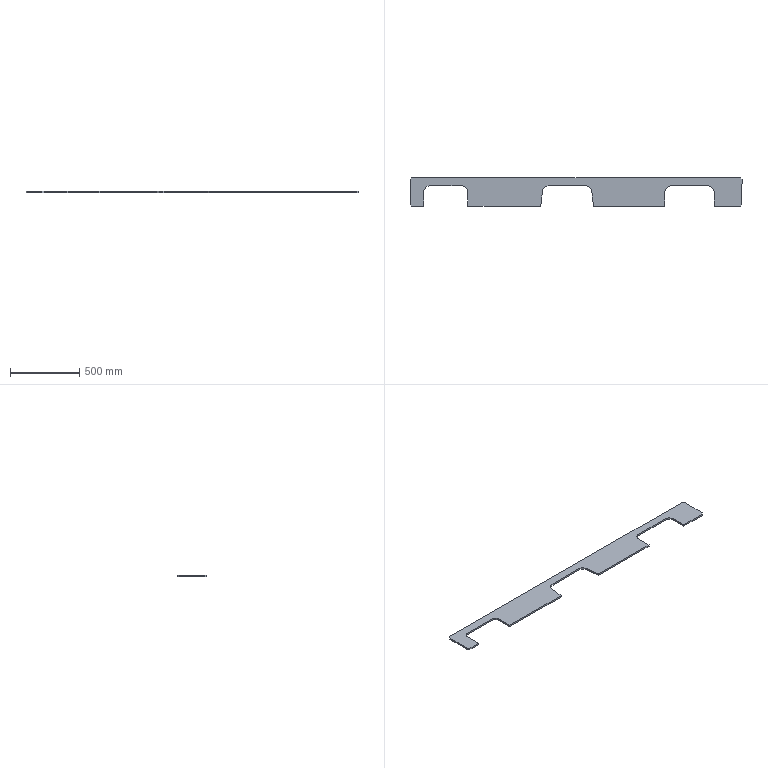Part | SolidWorks | features Extrusion 1 | 1 solid | 28 faces | box 2400 x 207 x 12 mm | volume 4150722 mm3 | plane 22 | cylinder 6 | commonest cylinder face diameters 80 x6
STEP:
#1=CARTESIAN_POINT('',(0.,12.,0.));
#2=VERTEX_POINT('',#1);
#3=CARTESIAN_POINT('',(12.,0.,0.));
#4=VERTEX_POINT('',#3);
#5=CARTESIAN_POINT('',(0.,12.,0.));
#6=DIRECTION('',(0.7071,-0.7071,0.));
#7=VECTOR('',#6,1000.);
#8=LINE('',#5,#7);
#9=EDGE_CURVE('',#2,#4,#8,.T.);
#10=ORIENTED_EDGE('',*,*,#9,.T.);
#11=CARTESIAN_POINT('',(12.,0.,12.));
#12=VERTEX_POINT('',#11);
#13=CARTESIAN_POINT('',(12.,0.,12.));
#14=DIRECTION('',(0.,0.,-1.));
#15=VECTOR('',#14,1000.);
#16=LINE('',#13,#15);
#17=EDGE_CURVE('',#12,#4,#16,.T.);
#18=ORIENTED_EDGE('',*,*,#17,.F.);
#19=CARTESIAN_POINT('',(0.,12.,12.));
#20=VERTEX_POINT('',#19);
#21=CARTESIAN_POINT('',(0.,12.,12.));
#22=DIRECTION('',(0.7071,-0.7071,0.));
#23=VECTOR('',#22,1000.);
#24=LINE('',#21,#23);
#25=EDGE_CURVE('',#20,#12,#24,.T.);
#26=ORIENTED_EDGE('',*,*,#25,.F.);
#27=CARTESIAN_POINT('',(0.,12.,12.));
#28=DIRECTION('',(0.,0.,-1.));
#29=VECTOR('',#28,1000.);
#30=LINE('',#27,#29);
#31=EDGE_CURVE('',#20,#2,#30,.T.);
#32=ORIENTED_EDGE('',*,*,#31,.T.);
#33=EDGE_LOOP('',(#10,#18,#26,#32));
#34=FACE_OUTER_BOUND('',#33,.T.);
#35=CARTESIAN_POINT('',(0.,12.,12.));
#36=DIRECTION('',(0.7071,0.7071,0.));
#37=DIRECTION('',(-0.7071,0.7071,0.));
#38=AXIS2_PLACEMENT_3D('',#35,#36,#37);
#39=PLANE('',#38);
#40=ADVANCED_FACE('',(#34),#39,.F.);
#41=CARTESIAN_POINT('',(100.,0.,0.));
#42=VERTEX_POINT('',#41);
#43=CARTESIAN_POINT('',(12.,0.,0.));
#44=DIRECTION('',(1.,0.,0.));
#45=VECTOR('',#44,1000.);
#46=LINE('',#43,#45);
#47=EDGE_CURVE('',#4,#42,#46,.T.);
#48=ORIENTED_EDGE('',*,*,#47,.T.);
#49=CARTESIAN_POINT('',(100.,0.,12.));
#50=VERTEX_POINT('',#49);
#51=CARTESIAN_POINT('',(100.,0.,12.));
#52=DIRECTION('',(0.,0.,-1.));
#53=VECTOR('',#52,1000.);
#54=LINE('',#51,#53);
#55=EDGE_CURVE('',#50,#42,#54,.T.);
#56=ORIENTED_EDGE('',*,*,#55,.F.);
#57=CARTESIAN_POINT('',(12.,0.,12.));
#58=DIRECTION('',(1.,0.,0.));
#59=VECTOR('',#58,1000.);
#60=LINE('',#57,#59);
#61=EDGE_CURVE('',#12,#50,#60,.T.);
#62=ORIENTED_EDGE('',*,*,#61,.F.);
#63=ORIENTED_EDGE('',*,*,#17,.T.);
#64=EDGE_LOOP('',(#48,#56,#62,#63));
#65=FACE_OUTER_BOUND('',#64,.T.);
#66=CARTESIAN_POINT('',(12.,0.,12.));
#67=DIRECTION('',(0.,1.,0.));
#68=DIRECTION('',(0.,0.,1.));
#69=AXIS2_PLACEMENT_3D('',#66,#67,#68);
#70=PLANE('',#69);
#71=ADVANCED_FACE('',(#65),#70,.F.);
#72=CARTESIAN_POINT('',(100.,107.,0.));
#73=VERTEX_POINT('',#72);
#74=CARTESIAN_POINT('',(100.,107.,0.));
#75=DIRECTION('',(0.,1.,0.));
#76=VECTOR('',#75,1000.);
#77=LINE('',#74,#76);
#78=EDGE_CURVE('',#42,#73,#77,.T.);
#79=ORIENTED_EDGE('',*,*,#78,.T.);
#80=CARTESIAN_POINT('',(100.,107.,12.));
#81=VERTEX_POINT('',#80);
#82=CARTESIAN_POINT('',(100.,107.,12.));
#83=DIRECTION('',(0.,0.,-1.));
#84=VECTOR('',#83,1000.);
#85=LINE('',#82,#84);
#86=EDGE_CURVE('',#81,#73,#85,.T.);
#87=ORIENTED_EDGE('',*,*,#86,.F.);
#88=CARTESIAN_POINT('',(100.,107.,12.));
#89=DIRECTION('',(0.,1.,0.));
#90=VECTOR('',#89,1000.);
#91=LINE('',#88,#90);
#92=EDGE_CURVE('',#50,#81,#91,.T.);
#93=ORIENTED_EDGE('',*,*,#92,.F.);
#94=ORIENTED_EDGE('',*,*,#55,.T.);
#95=EDGE_LOOP('',(#79,#87,#93,#94));
#96=FACE_OUTER_BOUND('',#95,.T.);
#97=CARTESIAN_POINT('',(100.,107.,12.));
#98=DIRECTION('',(-1.,0.,0.));
#99=DIRECTION('',(0.,-1.,0.));
#100=AXIS2_PLACEMENT_3D('',#97,#98,#99);
#101=PLANE('',#100);
#102=ADVANCED_FACE('',(#96),#101,.F.);
#103=CARTESIAN_POINT('',(140.,147.,0.));
#104=VERTEX_POINT('',#103);
#105=CARTESIAN_POINT('',(140.,107.,0.));
#106=DIRECTION('',(0.,0.,-1.));
#107=DIRECTION('',(-1.,0.,0.));
#108=AXIS2_PLACEMENT_3D('',#105,#106,#107);
#109=CIRCLE('',#108,40.);
#110=EDGE_CURVE('',#73,#104,#109,.T.);
#111=ORIENTED_EDGE('',*,*,#110,.T.);
#112=CARTESIAN_POINT('',(140.,147.,12.));
#113=VERTEX_POINT('',#112);
#114=CARTESIAN_POINT('',(140.,147.,12.));
#115=DIRECTION('',(0.,0.,-1.));
#116=VECTOR('',#115,1000.);
#117=LINE('',#114,#116);
#118=EDGE_CURVE('',#113,#104,#117,.T.);
#119=ORIENTED_EDGE('',*,*,#118,.F.);
#120=CARTESIAN_POINT('',(140.,107.,12.));
#121=DIRECTION('',(0.,0.,-1.));
#122=DIRECTION('',(-1.,0.,0.));
#123=AXIS2_PLACEMENT_3D('',#120,#121,#122);
#124=CIRCLE('',#123,40.);
#125=EDGE_CURVE('',#81,#113,#124,.T.);
#126=ORIENTED_EDGE('',*,*,#125,.F.);
#127=ORIENTED_EDGE('',*,*,#86,.T.);
#128=EDGE_LOOP('',(#111,#119,#126,#127));
#129=FACE_OUTER_BOUND('',#128,.T.);
#130=CARTESIAN_POINT('',(140.,107.,12.));
#131=DIRECTION('',(0.,0.,-1.));
#132=DIRECTION('',(-1.,0.,0.));
#133=AXIS2_PLACEMENT_3D('',#130,#131,#132);
#134=CYLINDRICAL_SURFACE('',#133,40.);
#135=ADVANCED_FACE('',(#129),#134,.F.);
#136=CARTESIAN_POINT('',(378.,147.,0.));
#137=VERTEX_POINT('',#136);
#138=CARTESIAN_POINT('',(140.,147.,0.));
#139=DIRECTION('',(1.,0.,0.));
#140=VECTOR('',#139,1000.);
#141=LINE('',#138,#140);
#142=EDGE_CURVE('',#104,#137,#141,.T.);
#143=ORIENTED_EDGE('',*,*,#142,.T.);
#144=CARTESIAN_POINT('',(378.,147.,12.));
#145=VERTEX_POINT('',#144);
#146=CARTESIAN_POINT('',(378.,147.,12.));
#147=DIRECTION('',(0.,0.,-1.));
#148=VECTOR('',#147,1000.);
#149=LINE('',#146,#148);
#150=EDGE_CURVE('',#145,#137,#149,.T.);
#151=ORIENTED_EDGE('',*,*,#150,.F.);
#152=CARTESIAN_POINT('',(140.,147.,12.));
#153=DIRECTION('',(1.,0.,0.));
#154=VECTOR('',#153,1000.);
#155=LINE('',#152,#154);
#156=EDGE_CURVE('',#113,#145,#155,.T.);
#157=ORIENTED_EDGE('',*,*,#156,.F.);
#158=ORIENTED_EDGE('',*,*,#118,.T.);
#159=EDGE_LOOP('',(#143,#151,#157,#158));
#160=FACE_OUTER_BOUND('',#159,.T.);
#161=CARTESIAN_POINT('',(140.,147.,12.));
#162=DIRECTION('',(0.,1.,0.));
#163=DIRECTION('',(-1.,0.,0.));
#164=AXIS2_PLACEMENT_3D('',#161,#162,#163);
#165=PLANE('',#164);
#166=ADVANCED_FACE('',(#160),#165,.F.);
#167=CARTESIAN_POINT('',(418.,107.,0.));
#168=VERTEX_POINT('',#167);
#169=CARTESIAN_POINT('',(378.,107.,0.));
#170=DIRECTION('',(0.,0.,-1.));
#171=DIRECTION('',(1.,0.,0.));
#172=AXIS2_PLACEMENT_3D('',#169,#170,#171);
#173=CIRCLE('',#172,40.);
#174=EDGE_CURVE('',#137,#168,#173,.T.);
#175=ORIENTED_EDGE('',*,*,#174,.T.);
#176=CARTESIAN_POINT('',(418.,107.,12.));
#177=VERTEX_POINT('',#176);
#178=CARTESIAN_POINT('',(418.,107.,12.));
#179=DIRECTION('',(0.,0.,-1.));
#180=VECTOR('',#179,1000.);
#181=LINE('',#178,#180);
#182=EDGE_CURVE('',#177,#168,#181,.T.);
#183=ORIENTED_EDGE('',*,*,#182,.F.);
#184=CARTESIAN_POINT('',(378.,107.,12.));
#185=DIRECTION('',(0.,0.,-1.));
#186=DIRECTION('',(1.,0.,0.));
#187=AXIS2_PLACEMENT_3D('',#184,#185,#186);
#188=CIRCLE('',#187,40.);
#189=EDGE_CURVE('',#145,#177,#188,.T.);
#190=ORIENTED_EDGE('',*,*,#189,.F.);
#191=ORIENTED_EDGE('',*,*,#150,.T.);
#192=EDGE_LOOP('',(#175,#183,#190,#191));
#193=FACE_OUTER_BOUND('',#192,.T.);
#194=CARTESIAN_POINT('',(378.,107.,12.));
#195=DIRECTION('',(0.,0.,-1.));
#196=DIRECTION('',(-1.,0.,0.));
#197=AXIS2_PLACEMENT_3D('',#194,#195,#196);
#198=CYLINDRICAL_SURFACE('',#197,40.);
#199=ADVANCED_FACE('',(#193),#198,.F.);
#200=CARTESIAN_POINT('',(418.,0.,0.));
#201=VERTEX_POINT('',#200);
#202=CARTESIAN_POINT('',(418.,107.,0.));
#203=DIRECTION('',(0.,-1.,0.));
#204=VECTOR('',#203,1000.);
#205=LINE('',#202,#204);
#206=EDGE_CURVE('',#168,#201,#205,.T.);
#207=ORIENTED_EDGE('',*,*,#206,.T.);
#208=CARTESIAN_POINT('',(418.,0.,12.));
#209=VERTEX_POINT('',#208);
#210=CARTESIAN_POINT('',(418.,0.,12.));
#211=DIRECTION('',(0.,0.,-1.));
#212=VECTOR('',#211,1000.);
#213=LINE('',#210,#212);
#214=EDGE_CURVE('',#209,#201,#213,.T.);
#215=ORIENTED_EDGE('',*,*,#214,.F.);
#216=CARTESIAN_POINT('',(418.,107.,12.));
#217=DIRECTION('',(0.,-1.,0.));
#218=VECTOR('',#217,1000.);
#219=LINE('',#216,#218);
#220=EDGE_CURVE('',#177,#209,#219,.T.);
#221=ORIENTED_EDGE('',*,*,#220,.F.);
#222=ORIENTED_EDGE('',*,*,#182,.T.);
#223=EDGE_LOOP('',(#207,#215,#221,#222));
#224=FACE_OUTER_BOUND('',#223,.T.);
#225=CARTESIAN_POINT('',(418.,107.,12.));
#226=DIRECTION('',(1.,0.,0.));
#227=DIRECTION('',(0.,0.,-1.));
#228=AXIS2_PLACEMENT_3D('',#225,#226,#227);
#229=PLANE('',#228);
#230=ADVANCED_FACE('',(#224),#229,.F.);
#231=CARTESIAN_POINT('',(944.5,0.,0.));
#232=VERTEX_POINT('',#231);
#233=CARTESIAN_POINT('',(418.,0.,0.));
#234=DIRECTION('',(1.,0.,0.));
#235=VECTOR('',#234,1000.);
#236=LINE('',#233,#235);
#237=EDGE_CURVE('',#201,#232,#236,.T.);
#238=ORIENTED_EDGE('',*,*,#237,.T.);
#239=CARTESIAN_POINT('',(944.5,0.,12.));
#240=VERTEX_POINT('',#239);
#241=CARTESIAN_POINT('',(944.5,0.,12.));
#242=DIRECTION('',(0.,0.,-1.));
#243=VECTOR('',#242,1000.);
#244=LINE('',#241,#243);
#245=EDGE_CURVE('',#240,#232,#244,.T.);
#246=ORIENTED_EDGE('',*,*,#245,.F.);
#247=CARTESIAN_POINT('',(418.,0.,12.));
#248=DIRECTION('',(1.,0.,0.));
#249=VECTOR('',#248,1000.);
#250=LINE('',#247,#249);
#251=EDGE_CURVE('',#209,#240,#250,.T.);
#252=ORIENTED_EDGE('',*,*,#251,.F.);
#253=ORIENTED_EDGE('',*,*,#214,.T.);
#254=EDGE_LOOP('',(#238,#246,#252,#253));
#255=FACE_OUTER_BOUND('',#254,.T.);
#256=CARTESIAN_POINT('',(418.,0.,12.));
#257=DIRECTION('',(0.,1.,0.));
#258=DIRECTION('',(0.,0.,1.));
#259=AXIS2_PLACEMENT_3D('',#256,#257,#258);
#260=PLANE('',#259);
#261=ADVANCED_FACE('',(#255),#260,.F.);
#262=CARTESIAN_POINT('',(958.236,111.875,0.));
#263=VERTEX_POINT('',#262);
#264=CARTESIAN_POINT('',(944.5,0.,0.));
#265=DIRECTION('',(0.1219,0.9925,0.));
#266=VECTOR('',#265,1000.);
#267=LINE('',#264,#266);
#268=EDGE_CURVE('',#232,#263,#267,.T.);
#269=ORIENTED_EDGE('',*,*,#268,.T.);
#270=CARTESIAN_POINT('',(958.236,111.875,12.));
#271=VERTEX_POINT('',#270);
#272=CARTESIAN_POINT('',(958.236,111.875,12.));
#273=DIRECTION('',(0.,0.,-1.));
#274=VECTOR('',#273,1000.);
#275=LINE('',#272,#274);
#276=EDGE_CURVE('',#271,#263,#275,.T.);
#277=ORIENTED_EDGE('',*,*,#276,.F.);
#278=CARTESIAN_POINT('',(944.5,0.,12.));
#279=DIRECTION('',(0.1219,0.9925,0.));
#280=VECTOR('',#279,1000.);
#281=LINE('',#278,#280);
#282=EDGE_CURVE('',#240,#271,#281,.T.);
#283=ORIENTED_EDGE('',*,*,#282,.F.);
#284=ORIENTED_EDGE('',*,*,#245,.T.);
#285=EDGE_LOOP('',(#269,#277,#283,#284));
#286=FACE_OUTER_BOUND('',#285,.T.);
#287=CARTESIAN_POINT('',(944.5,0.,12.));
#288=DIRECTION('',(-0.9925,0.1219,0.));
#289=DIRECTION('',(-0.1219,-0.9925,0.));
#290=AXIS2_PLACEMENT_3D('',#287,#288,#289);
#291=PLANE('',#290);
#292=ADVANCED_FACE('',(#286),#291,.F.);
#293=CARTESIAN_POINT('',(997.938,147.,0.));
#294=VERTEX_POINT('',#293);
#295=CARTESIAN_POINT('',(997.938,107.,0.));
#296=DIRECTION('',(0.,0.,-1.));
#297=DIRECTION('',(-1.,0.,0.));
#298=AXIS2_PLACEMENT_3D('',#295,#296,#297);
#299=CIRCLE('',#298,40.);
#300=EDGE_CURVE('',#263,#294,#299,.T.);
#301=ORIENTED_EDGE('',*,*,#300,.T.);
#302=CARTESIAN_POINT('',(997.938,147.,12.));
#303=VERTEX_POINT('',#302);
#304=CARTESIAN_POINT('',(997.938,147.,12.));
#305=DIRECTION('',(0.,0.,-1.));
#306=VECTOR('',#305,1000.);
#307=LINE('',#304,#306);
#308=EDGE_CURVE('',#303,#294,#307,.T.);
#309=ORIENTED_EDGE('',*,*,#308,.F.);
#310=CARTESIAN_POINT('',(997.938,107.,12.));
#311=DIRECTION('',(0.,0.,-1.));
#312=DIRECTION('',(-1.,0.,0.));
#313=AXIS2_PLACEMENT_3D('',#310,#311,#312);
#314=CIRCLE('',#313,40.);
#315=EDGE_CURVE('',#271,#303,#314,.T.);
#316=ORIENTED_EDGE('',*,*,#315,.F.);
#317=ORIENTED_EDGE('',*,*,#276,.T.);
#318=EDGE_LOOP('',(#301,#309,#316,#317));
#319=FACE_OUTER_BOUND('',#318,.T.);
#320=CARTESIAN_POINT('',(997.938,107.,12.));
#321=DIRECTION('',(0.,0.,-1.));
#322=DIRECTION('',(-1.,0.,0.));
#323=AXIS2_PLACEMENT_3D('',#320,#321,#322);
#324=CYLINDRICAL_SURFACE('',#323,40.);
#325=ADVANCED_FACE('',(#319),#324,.F.);
#326=CARTESIAN_POINT('',(1273.562,147.,0.));
#327=VERTEX_POINT('',#326);
#328=CARTESIAN_POINT('',(997.938,147.,0.));
#329=DIRECTION('',(1.,0.,0.));
#330=VECTOR('',#329,1000.);
#331=LINE('',#328,#330);
#332=EDGE_CURVE('',#294,#327,#331,.T.);
#333=ORIENTED_EDGE('',*,*,#332,.T.);
#334=CARTESIAN_POINT('',(1273.562,147.,12.));
#335=VERTEX_POINT('',#334);
#336=CARTESIAN_POINT('',(1273.562,147.,12.));
#337=DIRECTION('',(0.,0.,-1.));
#338=VECTOR('',#337,1000.);
#339=LINE('',#336,#338);
#340=EDGE_CURVE('',#335,#327,#339,.T.);
#341=ORIENTED_EDGE('',*,*,#340,.F.);
#342=CARTESIAN_POINT('',(997.938,147.,12.));
#343=DIRECTION('',(1.,0.,0.));
#344=VECTOR('',#343,1000.);
#345=LINE('',#342,#344);
#346=EDGE_CURVE('',#303,#335,#345,.T.);
#347=ORIENTED_EDGE('',*,*,#346,.F.);
#348=ORIENTED_EDGE('',*,*,#308,.T.);
#349=EDGE_LOOP('',(#333,#341,#347,#348));
#350=FACE_OUTER_BOUND('',#349,.T.);
#351=CARTESIAN_POINT('',(997.938,147.,12.));
#352=DIRECTION('',(0.,1.,0.));
#353=DIRECTION('',(-1.,0.,0.));
#354=AXIS2_PLACEMENT_3D('',#351,#352,#353);
#355=PLANE('',#354);
#356=ADVANCED_FACE('',(#350),#355,.F.);
#357=CARTESIAN_POINT('',(1313.264,111.875,0.));
#358=VERTEX_POINT('',#357);
#359=CARTESIAN_POINT('',(1273.562,107.,0.));
#360=DIRECTION('',(0.,0.,-1.));
#361=DIRECTION('',(1.,0.,0.));
#362=AXIS2_PLACEMENT_3D('',#359,#360,#361);
#363=CIRCLE('',#362,40.);
#364=EDGE_CURVE('',#327,#358,#363,.T.);
#365=ORIENTED_EDGE('',*,*,#364,.T.);
#366=CARTESIAN_POINT('',(1313.264,111.875,12.));
#367=VERTEX_POINT('',#366);
#368=CARTESIAN_POINT('',(1313.264,111.875,12.));
#369=DIRECTION('',(0.,0.,-1.));
#370=VECTOR('',#369,1000.);
#371=LINE('',#368,#370);
#372=EDGE_CURVE('',#367,#358,#371,.T.);
#373=ORIENTED_EDGE('',*,*,#372,.F.);
#374=CARTESIAN_POINT('',(1273.562,107.,12.));
#375=DIRECTION('',(0.,0.,-1.));
#376=DIRECTION('',(1.,0.,0.));
#377=AXIS2_PLACEMENT_3D('',#374,#375,#376);
#378=CIRCLE('',#377,40.);
#379=EDGE_CURVE('',#335,#367,#378,.T.);
#380=ORIENTED_EDGE('',*,*,#379,.F.);
#381=ORIENTED_EDGE('',*,*,#340,.T.);
#382=EDGE_LOOP('',(#365,#373,#380,#381));
#383=FACE_OUTER_BOUND('',#382,.T.);
#384=CARTESIAN_POINT('',(1273.562,107.,12.));
#385=DIRECTION('',(0.,0.,-1.));
#386=DIRECTION('',(-1.,0.,0.));
#387=AXIS2_PLACEMENT_3D('',#384,#385,#386);
#388=CYLINDRICAL_SURFACE('',#387,40.);
#389=ADVANCED_FACE('',(#383),#388,.F.);
#390=CARTESIAN_POINT('',(1327.,0.,0.));
#391=VERTEX_POINT('',#390);
#392=CARTESIAN_POINT('',(1327.,0.,0.));
#393=DIRECTION('',(0.1219,-0.9925,0.));
#394=VECTOR('',#393,1000.);
#395=LINE('',#392,#394);
#396=EDGE_CURVE('',#358,#391,#395,.T.);
#397=ORIENTED_EDGE('',*,*,#396,.T.);
#398=CARTESIAN_POINT('',(1327.,0.,12.));
#399=VERTEX_POINT('',#398);
#400=CARTESIAN_POINT('',(1327.,0.,12.));
#401=DIRECTION('',(0.,0.,-1.));
#402=VECTOR('',#401,1000.);
#403=LINE('',#400,#402);
#404=EDGE_CURVE('',#399,#391,#403,.T.);
#405=ORIENTED_EDGE('',*,*,#404,.F.);
#406=CARTESIAN_POINT('',(1327.,0.,12.));
#407=DIRECTION('',(0.1219,-0.9925,0.));
#408=VECTOR('',#407,1000.);
#409=LINE('',#406,#408);
#410=EDGE_CURVE('',#367,#399,#409,.T.);
#411=ORIENTED_EDGE('',*,*,#410,.F.);
#412=ORIENTED_EDGE('',*,*,#372,.T.);
#413=EDGE_LOOP('',(#397,#405,#411,#412));
#414=FACE_OUTER_BOUND('',#413,.T.);
#415=CARTESIAN_POINT('',(1327.,0.,12.));
#416=DIRECTION('',(0.9925,0.1219,0.));
#417=DIRECTION('',(-0.1219,0.9925,0.));
#418=AXIS2_PLACEMENT_3D('',#415,#416,#417);
#419=PLANE('',#418);
#420=ADVANCED_FACE('',(#414),#419,.F.);
#421=CARTESIAN_POINT('',(1843.,0.,0.));
#422=VERTEX_POINT('',#421);
#423=CARTESIAN_POINT('',(1327.,0.,0.));
#424=DIRECTION('',(1.,0.,0.));
#425=VECTOR('',#424,1000.);
#426=LINE('',#423,#425);
#427=EDGE_CURVE('',#391,#422,#426,.T.);
#428=ORIENTED_EDGE('',*,*,#427,.T.);
#429=CARTESIAN_POINT('',(1843.,0.,12.));
#430=VERTEX_POINT('',#429);
#431=CARTESIAN_POINT('',(1843.,0.,12.));
#432=DIRECTION('',(0.,0.,-1.));
#433=VECTOR('',#432,1000.);
#434=LINE('',#431,#433);
#435=EDGE_CURVE('',#430,#422,#434,.T.);
#436=ORIENTED_EDGE('',*,*,#435,.F.);
#437=CARTESIAN_POINT('',(1327.,0.,12.));
#438=DIRECTION('',(1.,0.,0.));
#439=VECTOR('',#438,1000.);
#440=LINE('',#437,#439);
#441=EDGE_CURVE('',#399,#430,#440,.T.);
#442=ORIENTED_EDGE('',*,*,#441,.F.);
#443=ORIENTED_EDGE('',*,*,#404,.T.);
#444=EDGE_LOOP('',(#428,#436,#442,#443));
#445=FACE_OUTER_BOUND('',#444,.T.);
#446=CARTESIAN_POINT('',(1327.,0.,12.));
#447=DIRECTION('',(0.,1.,0.));
#448=DIRECTION('',(-1.,0.,0.));
#449=AXIS2_PLACEMENT_3D('',#446,#447,#448);
#450=PLANE('',#449);
#451=ADVANCED_FACE('',(#445),#450,.F.);
#452=CARTESIAN_POINT('',(1843.,107.,0.));
#453=VERTEX_POINT('',#452);
#454=CARTESIAN_POINT('',(1843.,107.,0.));
#455=DIRECTION('',(0.,1.,0.));
#456=VECTOR('',#455,1000.);
#457=LINE('',#454,#456);
#458=EDGE_CURVE('',#422,#453,#457,.T.);
#459=ORIENTED_EDGE('',*,*,#458,.T.);
#460=CARTESIAN_POINT('',(1843.,107.,12.));
#461=VERTEX_POINT('',#460);
#462=CARTESIAN_POINT('',(1843.,107.,12.));
#463=DIRECTION('',(0.,0.,-1.));
#464=VECTOR('',#463,1000.);
#465=LINE('',#462,#464);
#466=EDGE_CURVE('',#461,#453,#465,.T.);
#467=ORIENTED_EDGE('',*,*,#466,.F.);
#468=CARTESIAN_POINT('',(1843.,107.,12.));
#469=DIRECTION('',(0.,1.,0.));
#470=VECTOR('',#469,1000.);
#471=LINE('',#468,#470);
#472=EDGE_CURVE('',#430,#461,#471,.T.);
#473=ORIENTED_EDGE('',*,*,#472,.F.);
#474=ORIENTED_EDGE('',*,*,#435,.T.);
#475=EDGE_LOOP('',(#459,#467,#473,#474));
#476=FACE_OUTER_BOUND('',#475,.T.);
#477=CARTESIAN_POINT('',(1843.,107.,12.));
#478=DIRECTION('',(-1.,0.,0.));
#479=DIRECTION('',(0.,0.,1.));
#480=AXIS2_PLACEMENT_3D('',#477,#478,#479);
#481=PLANE('',#480);
#482=ADVANCED_FACE('',(#476),#481,.F.);
#483=CARTESIAN_POINT('',(1883.,147.,0.));
#484=VERTEX_POINT('',#483);
#485=CARTESIAN_POINT('',(1883.,107.,0.));
#486=DIRECTION('',(0.,0.,-1.));
#487=DIRECTION('',(-1.,0.,0.));
#488=AXIS2_PLACEMENT_3D('',#485,#486,#487);
#489=CIRCLE('',#488,40.);
#490=EDGE_CURVE('',#453,#484,#489,.T.);
#491=ORIENTED_EDGE('',*,*,#490,.T.);
#492=CARTESIAN_POINT('',(1883.,147.,12.));
#493=VERTEX_POINT('',#492);
#494=CARTESIAN_POINT('',(1883.,147.,12.));
#495=DIRECTION('',(0.,0.,-1.));
#496=VECTOR('',#495,1000.);
#497=LINE('',#494,#496);
#498=EDGE_CURVE('',#493,#484,#497,.T.);
#499=ORIENTED_EDGE('',*,*,#498,.F.);
#500=CARTESIAN_POINT('',(1883.,107.,12.));
#501=DIRECTION('',(0.,0.,-1.));
#502=DIRECTION('',(-1.,0.,0.));
#503=AXIS2_PLACEMENT_3D('',#500,#501,#502);
#504=CIRCLE('',#503,40.);
#505=EDGE_CURVE('',#461,#493,#504,.T.);
#506=ORIENTED_EDGE('',*,*,#505,.F.);
#507=ORIENTED_EDGE('',*,*,#466,.T.);
#508=EDGE_LOOP('',(#491,#499,#506,#507));
#509=FACE_OUTER_BOUND('',#508,.T.);
#510=CARTESIAN_POINT('',(1883.,107.,12.));
#511=DIRECTION('',(0.,0.,-1.));
#512=DIRECTION('',(-1.,0.,0.));
#513=AXIS2_PLACEMENT_3D('',#510,#511,#512);
#514=CYLINDRICAL_SURFACE('',#513,40.);
#515=ADVANCED_FACE('',(#509),#514,.F.);
#516=CARTESIAN_POINT('',(2158.,147.,0.));
#517=VERTEX_POINT('',#516);
#518=CARTESIAN_POINT('',(1883.,147.,0.));
#519=DIRECTION('',(1.,0.,0.));
#520=VECTOR('',#519,1000.);
#521=LINE('',#518,#520);
#522=EDGE_CURVE('',#484,#517,#521,.T.);
#523=ORIENTED_EDGE('',*,*,#522,.T.);
#524=CARTESIAN_POINT('',(2158.,147.,12.));
#525=VERTEX_POINT('',#524);
#526=CARTESIAN_POINT('',(2158.,147.,12.));
#527=DIRECTION('',(0.,0.,-1.));
#528=VECTOR('',#527,1000.);
#529=LINE('',#526,#528);
#530=EDGE_CURVE('',#525,#517,#529,.T.);
#531=ORIENTED_EDGE('',*,*,#530,.F.);
#532=CARTESIAN_POINT('',(1883.,147.,12.));
#533=DIRECTION('',(1.,0.,0.));
#534=VECTOR('',#533,1000.);
#535=LINE('',#532,#534);
#536=EDGE_CURVE('',#493,#525,#535,.T.);
#537=ORIENTED_EDGE('',*,*,#536,.F.);
#538=ORIENTED_EDGE('',*,*,#498,.T.);
#539=EDGE_LOOP('',(#523,#531,#537,#538));
#540=FACE_OUTER_BOUND('',#539,.T.);
#541=CARTESIAN_POINT('',(1883.,147.,12.));
#542=DIRECTION('',(0.,1.,0.));
#543=DIRECTION('',(-1.,0.,0.));
#544=AXIS2_PLACEMENT_3D('',#541,#542,#543);
#545=PLANE('',#544);
#546=ADVANCED_FACE('',(#540),#545,.F.);
#547=CARTESIAN_POINT('',(2198.,107.,0.));
#548=VERTEX_POINT('',#547);
#549=CARTESIAN_POINT('',(2158.,107.,0.));
#550=DIRECTION('',(0.,0.,-1.));
#551=DIRECTION('',(1.,0.,0.));
#552=AXIS2_PLACEMENT_3D('',#549,#550,#551);
#553=CIRCLE('',#552,40.);
#554=EDGE_CURVE('',#517,#548,#553,.T.);
#555=ORIENTED_EDGE('',*,*,#554,.T.);
#556=CARTESIAN_POINT('',(2198.,107.,12.));
#557=VERTEX_POINT('',#556);
#558=CARTESIAN_POINT('',(2198.,107.,12.));
#559=DIRECTION('',(0.,0.,-1.));
#560=VECTOR('',#559,1000.);
#561=LINE('',#558,#560);
#562=EDGE_CURVE('',#557,#548,#561,.T.);
#563=ORIENTED_EDGE('',*,*,#562,.F.);
#564=CARTESIAN_POINT('',(2158.,107.,12.));
#565=DIRECTION('',(0.,0.,-1.));
#566=DIRECTION('',(1.,0.,0.));
#567=AXIS2_PLACEMENT_3D('',#564,#565,#566);
#568=CIRCLE('',#567,40.);
#569=EDGE_CURVE('',#525,#557,#568,.T.);
#570=ORIENTED_EDGE('',*,*,#569,.F.);
#571=ORIENTED_EDGE('',*,*,#530,.T.);
#572=EDGE_LOOP('',(#555,#563,#570,#571));
#573=FACE_OUTER_BOUND('',#572,.T.);
#574=CARTESIAN_POINT('',(2158.,107.,12.));
#575=DIRECTION('',(0.,0.,-1.));
#576=DIRECTION('',(-1.,0.,0.));
#577=AXIS2_PLACEMENT_3D('',#574,#575,#576);
#578=CYLINDRICAL_SURFACE('',#577,40.);
#579=ADVANCED_FACE('',(#573),#578,.F.);
#580=CARTESIAN_POINT('',(2198.,0.,0.));
#581=VERTEX_POINT('',#580);
#582=CARTESIAN_POINT('',(2198.,107.,0.));
#583=DIRECTION('',(0.,-1.,0.));
#584=VECTOR('',#583,1000.);
#585=LINE('',#582,#584);
#586=EDGE_CURVE('',#548,#581,#585,.T.);
#587=ORIENTED_EDGE('',*,*,#586,.T.);
#588=CARTESIAN_POINT('',(2198.,0.,12.));
#589=VERTEX_POINT('',#588);
#590=CARTESIAN_POINT('',(2198.,0.,12.));
#591=DIRECTION('',(0.,0.,-1.));
#592=VECTOR('',#591,1000.);
#593=LINE('',#590,#592);
#594=EDGE_CURVE('',#589,#581,#593,.T.);
#595=ORIENTED_EDGE('',*,*,#594,.F.);
#596=CARTESIAN_POINT('',(2198.,107.,12.));
#597=DIRECTION('',(0.,-1.,0.));
#598=VECTOR('',#597,1000.);
#599=LINE('',#596,#598);
#600=EDGE_CURVE('',#557,#589,#599,.T.);
#601=ORIENTED_EDGE('',*,*,#600,.F.);
#602=ORIENTED_EDGE('',*,*,#562,.T.);
#603=EDGE_LOOP('',(#587,#595,#601,#602));
#604=FACE_OUTER_BOUND('',#603,.T.);
#605=CARTESIAN_POINT('',(2198.,107.,12.));
#606=DIRECTION('',(1.,0.,0.));
#607=DIRECTION('',(0.,0.,-1.));
#608=AXIS2_PLACEMENT_3D('',#605,#606,#607);
#609=PLANE('',#608);
#610=ADVANCED_FACE('',(#604),#609,.F.);
#611=CARTESIAN_POINT('',(2388.,0.,0.));
#612=VERTEX_POINT('',#611);
#613=CARTESIAN_POINT('',(2198.,0.,0.));
#614=DIRECTION('',(1.,0.,0.));
#615=VECTOR('',#614,1000.);
#616=LINE('',#613,#615);
#617=EDGE_CURVE('',#581,#612,#616,.T.);
#618=ORIENTED_EDGE('',*,*,#617,.T.);
#619=CARTESIAN_POINT('',(2388.,0.,12.));
#620=VERTEX_POINT('',#619);
#621=CARTESIAN_POINT('',(2388.,0.,12.));
#622=DIRECTION('',(0.,0.,-1.));
#623=VECTOR('',#622,1000.);
#624=LINE('',#621,#623);
#625=EDGE_CURVE('',#620,#612,#624,.T.);
#626=ORIENTED_EDGE('',*,*,#625,.F.);
#627=CARTESIAN_POINT('',(2198.,0.,12.));
#628=DIRECTION('',(1.,0.,0.));
#629=VECTOR('',#628,1000.);
#630=LINE('',#627,#629);
#631=EDGE_CURVE('',#589,#620,#630,.T.);
#632=ORIENTED_EDGE('',*,*,#631,.F.);
#633=ORIENTED_EDGE('',*,*,#594,.T.);
#634=EDGE_LOOP('',(#618,#626,#632,#633));
#635=FACE_OUTER_BOUND('',#634,.T.);
#636=CARTESIAN_POINT('',(2198.,0.,12.));
#637=DIRECTION('',(0.,1.,0.));
#638=DIRECTION('',(0.,0.,1.));
#639=AXIS2_PLACEMENT_3D('',#636,#637,#638);
#640=PLANE('',#639);
#641=ADVANCED_FACE('',(#635),#640,.F.);
#642=CARTESIAN_POINT('',(2400.,12.,0.));
#643=VERTEX_POINT('',#642);
#644=CARTESIAN_POINT('',(2388.,0.,0.));
#645=DIRECTION('',(0.7071,0.7071,0.));
#646=VECTOR('',#645,1000.);
#647=LINE('',#644,#646);
#648=EDGE_CURVE('',#612,#643,#647,.T.);
#649=ORIENTED_EDGE('',*,*,#648,.T.);
#650=CARTESIAN_POINT('',(2400.,12.,12.));
#651=VERTEX_POINT('',#650);
#652=CARTESIAN_POINT('',(2400.,12.,12.));
#653=DIRECTION('',(0.,0.,-1.));
#654=VECTOR('',#653,1000.);
#655=LINE('',#652,#654);
#656=EDGE_CURVE('',#651,#643,#655,.T.);
#657=ORIENTED_EDGE('',*,*,#656,.F.);
#658=CARTESIAN_POINT('',(2388.,0.,12.));
#659=DIRECTION('',(0.7071,0.7071,0.));
#660=VECTOR('',#659,1000.);
#661=LINE('',#658,#660);
#662=EDGE_CURVE('',#620,#651,#661,.T.);
#663=ORIENTED_EDGE('',*,*,#662,.F.);
#664=ORIENTED_EDGE('',*,*,#625,.T.);
#665=EDGE_LOOP('',(#649,#657,#663,#664));
#666=FACE_OUTER_BOUND('',#665,.T.);
#667=CARTESIAN_POINT('',(2388.,0.,12.));
#668=DIRECTION('',(-0.7071,0.7071,0.));
#669=DIRECTION('',(-0.7071,-0.7071,0.));
#670=AXIS2_PLACEMENT_3D('',#667,#668,#669);
#671=PLANE('',#670);
#672=ADVANCED_FACE('',(#666),#671,.F.);
#673=CARTESIAN_POINT('',(2400.,195.,0.));
#674=VERTEX_POINT('',#673);
#675=CARTESIAN_POINT('',(2400.,12.,0.));
#676=DIRECTION('',(0.,1.,0.));
#677=VECTOR('',#676,1000.);
#678=LINE('',#675,#677);
#679=EDGE_CURVE('',#643,#674,#678,.T.);
#680=ORIENTED_EDGE('',*,*,#679,.T.);
#681=CARTESIAN_POINT('',(2400.,195.,12.));
#682=VERTEX_POINT('',#681);
#683=CARTESIAN_POINT('',(2400.,195.,12.));
#684=DIRECTION('',(0.,0.,-1.));
#685=VECTOR('',#684,1000.);
#686=LINE('',#683,#685);
#687=EDGE_CURVE('',#682,#674,#686,.T.);
#688=ORIENTED_EDGE('',*,*,#687,.F.);
#689=CARTESIAN_POINT('',(2400.,12.,12.));
#690=DIRECTION('',(0.,1.,0.));
#691=VECTOR('',#690,1000.);
#692=LINE('',#689,#691);
#693=EDGE_CURVE('',#651,#682,#692,.T.);
#694=ORIENTED_EDGE('',*,*,#693,.F.);
#695=ORIENTED_EDGE('',*,*,#656,.T.);
#696=EDGE_LOOP('',(#680,#688,#694,#695));
#697=FACE_OUTER_BOUND('',#696,.T.);
#698=CARTESIAN_POINT('',(2400.,12.,12.));
#699=DIRECTION('',(-1.,0.,0.));
#700=DIRECTION('',(0.,-1.,0.));
#701=AXIS2_PLACEMENT_3D('',#698,#699,#700);
#702=PLANE('',#701);
#703=ADVANCED_FACE('',(#697),#702,.F.);
#704=CARTESIAN_POINT('',(2388.,207.,0.));
#705=VERTEX_POINT('',#704);
#706=CARTESIAN_POINT('',(2400.,195.,0.));
#707=DIRECTION('',(-0.7071,0.7071,0.));
#708=VECTOR('',#707,1000.);
#709=LINE('',#706,#708);
#710=EDGE_CURVE('',#674,#705,#709,.T.);
#711=ORIENTED_EDGE('',*,*,#710,.T.);
#712=CARTESIAN_POINT('',(2388.,207.,12.));
#713=VERTEX_POINT('',#712);
#714=CARTESIAN_POINT('',(2388.,207.,12.));
#715=DIRECTION('',(0.,0.,-1.));
#716=VECTOR('',#715,1000.);
#717=LINE('',#714,#716);
#718=EDGE_CURVE('',#713,#705,#717,.T.);
#719=ORIENTED_EDGE('',*,*,#718,.F.);
#720=CARTESIAN_POINT('',(2400.,195.,12.));
#721=DIRECTION('',(-0.7071,0.7071,0.));
#722=VECTOR('',#721,1000.);
#723=LINE('',#720,#722);
#724=EDGE_CURVE('',#682,#713,#723,.T.);
#725=ORIENTED_EDGE('',*,*,#724,.F.);
#726=ORIENTED_EDGE('',*,*,#687,.T.);
#727=EDGE_LOOP('',(#711,#719,#725,#726));
#728=FACE_OUTER_BOUND('',#727,.T.);
#729=CARTESIAN_POINT('',(2400.,195.,12.));
#730=DIRECTION('',(-0.7071,-0.7071,0.));
#731=DIRECTION('',(0.7071,-0.7071,0.));
#732=AXIS2_PLACEMENT_3D('',#729,#730,#731);
#733=PLANE('',#732);
#734=ADVANCED_FACE('',(#728),#733,.F.);
#735=CARTESIAN_POINT('',(12.,207.,0.));
#736=VERTEX_POINT('',#735);
#737=CARTESIAN_POINT('',(12.,207.,0.));
#738=DIRECTION('',(-1.,0.,0.));
#739=VECTOR('',#738,1000.);
#740=LINE('',#737,#739);
#741=EDGE_CURVE('',#705,#736,#740,.T.);
#742=ORIENTED_EDGE('',*,*,#741,.T.);
#743=CARTESIAN_POINT('',(12.,207.,12.));
#744=VERTEX_POINT('',#743);
#745=CARTESIAN_POINT('',(12.,207.,12.));
#746=DIRECTION('',(0.,0.,-1.));
#747=VECTOR('',#746,1000.);
#748=LINE('',#745,#747);
#749=EDGE_CURVE('',#744,#736,#748,.T.);
#750=ORIENTED_EDGE('',*,*,#749,.F.);
#751=CARTESIAN_POINT('',(12.,207.,12.));
#752=DIRECTION('',(-1.,0.,0.));
#753=VECTOR('',#752,1000.);
#754=LINE('',#751,#753);
#755=EDGE_CURVE('',#713,#744,#754,.T.);
#756=ORIENTED_EDGE('',*,*,#755,.F.);
#757=ORIENTED_EDGE('',*,*,#718,.T.);
#758=EDGE_LOOP('',(#742,#750,#756,#757));
#759=FACE_OUTER_BOUND('',#758,.T.);
#760=CARTESIAN_POINT('',(12.,207.,12.));
#761=DIRECTION('',(0.,-1.,0.));
#762=DIRECTION('',(0.,0.,-1.));
#763=AXIS2_PLACEMENT_3D('',#760,#761,#762);
#764=PLANE('',#763);
#765=ADVANCED_FACE('',(#759),#764,.F.);
#766=CARTESIAN_POINT('',(0.,195.,0.));
#767=VERTEX_POINT('',#766);
#768=CARTESIAN_POINT('',(0.,195.,0.));
#769=DIRECTION('',(-0.7071,-0.7071,0.));
#770=VECTOR('',#769,1000.);
#771=LINE('',#768,#770);
#772=EDGE_CURVE('',#736,#767,#771,.T.);
#773=ORIENTED_EDGE('',*,*,#772,.T.);
#774=CARTESIAN_POINT('',(0.,195.,12.));
#775=VERTEX_POINT('',#774);
#776=CARTESIAN_POINT('',(0.,195.,12.));
#777=DIRECTION('',(0.,0.,-1.));
#778=VECTOR('',#777,1000.);
#779=LINE('',#776,#778);
#780=EDGE_CURVE('',#775,#767,#779,.T.);
#781=ORIENTED_EDGE('',*,*,#780,.F.);
#782=CARTESIAN_POINT('',(0.,195.,12.));
#783=DIRECTION('',(-0.7071,-0.7071,0.));
#784=VECTOR('',#783,1000.);
#785=LINE('',#782,#784);
#786=EDGE_CURVE('',#744,#775,#785,.T.);
#787=ORIENTED_EDGE('',*,*,#786,.F.);
#788=ORIENTED_EDGE('',*,*,#749,.T.);
#789=EDGE_LOOP('',(#773,#781,#787,#788));
#790=FACE_OUTER_BOUND('',#789,.T.);
#791=CARTESIAN_POINT('',(0.,195.,12.));
#792=DIRECTION('',(0.7071,-0.7071,0.));
#793=DIRECTION('',(0.7071,0.7071,0.));
#794=AXIS2_PLACEMENT_3D('',#791,#792,#793);
#795=PLANE('',#794);
#796=ADVANCED_FACE('',(#790),#795,.F.);
#797=CARTESIAN_POINT('',(0.,12.,0.));
#798=DIRECTION('',(0.,-1.,0.));
#799=VECTOR('',#798,1000.);
#800=LINE('',#797,#799);
#801=EDGE_CURVE('',#767,#2,#800,.T.);
#802=ORIENTED_EDGE('',*,*,#801,.T.);
#803=ORIENTED_EDGE('',*,*,#31,.F.);
#804=CARTESIAN_POINT('',(0.,12.,12.));
#805=DIRECTION('',(0.,-1.,0.));
#806=VECTOR('',#805,1000.);
#807=LINE('',#804,#806);
#808=EDGE_CURVE('',#775,#20,#807,.T.);
#809=ORIENTED_EDGE('',*,*,#808,.F.);
#810=ORIENTED_EDGE('',*,*,#780,.T.);
#811=EDGE_LOOP('',(#802,#803,#809,#810));
#812=FACE_OUTER_BOUND('',#811,.T.);
#813=CARTESIAN_POINT('',(0.,12.,12.));
#814=DIRECTION('',(1.,0.,0.));
#815=DIRECTION('',(0.,0.,-1.));
#816=AXIS2_PLACEMENT_3D('',#813,#814,#815);
#817=PLANE('',#816);
#818=ADVANCED_FACE('',(#812),#817,.F.);
#819=ORIENTED_EDGE('',*,*,#25,.T.);
#820=ORIENTED_EDGE('',*,*,#61,.T.);
#821=ORIENTED_EDGE('',*,*,#92,.T.);
#822=ORIENTED_EDGE('',*,*,#125,.T.);
#823=ORIENTED_EDGE('',*,*,#156,.T.);
#824=ORIENTED_EDGE('',*,*,#189,.T.);
#825=ORIENTED_EDGE('',*,*,#220,.T.);
#826=ORIENTED_EDGE('',*,*,#251,.T.);
#827=ORIENTED_EDGE('',*,*,#282,.T.);
#828=ORIENTED_EDGE('',*,*,#315,.T.);
#829=ORIENTED_EDGE('',*,*,#346,.T.);
#830=ORIENTED_EDGE('',*,*,#379,.T.);
#831=ORIENTED_EDGE('',*,*,#410,.T.);
#832=ORIENTED_EDGE('',*,*,#441,.T.);
#833=ORIENTED_EDGE('',*,*,#472,.T.);
#834=ORIENTED_EDGE('',*,*,#505,.T.);
#835=ORIENTED_EDGE('',*,*,#536,.T.);
#836=ORIENTED_EDGE('',*,*,#569,.T.);
#837=ORIENTED_EDGE('',*,*,#600,.T.);
#838=ORIENTED_EDGE('',*,*,#631,.T.);
#839=ORIENTED_EDGE('',*,*,#662,.T.);
#840=ORIENTED_EDGE('',*,*,#693,.T.);
#841=ORIENTED_EDGE('',*,*,#724,.T.);
#842=ORIENTED_EDGE('',*,*,#755,.T.);
#843=ORIENTED_EDGE('',*,*,#786,.T.);
#844=ORIENTED_EDGE('',*,*,#808,.T.);
#845=EDGE_LOOP('',(#819,#820,#821,#822,#823,#824,#825,#826,#827,#828,#829,#830,#831,#832,#833,#834,#835,#836,#837,#838,#839,#840,#841,#842,#843,#844));
#846=FACE_OUTER_BOUND('',#845,.T.);
#847=CARTESIAN_POINT('',(140.,107.,12.));
#848=DIRECTION('',(0.,0.,-1.));
#849=DIRECTION('',(-1.,0.,0.));
#850=AXIS2_PLACEMENT_3D('',#847,#848,#849);
#851=PLANE('',#850);
#852=ADVANCED_FACE('',(#846),#851,.F.);
#853=ORIENTED_EDGE('',*,*,#9,.F.);
#854=ORIENTED_EDGE('',*,*,#801,.F.);
#855=ORIENTED_EDGE('',*,*,#772,.F.);
#856=ORIENTED_EDGE('',*,*,#741,.F.);
#857=ORIENTED_EDGE('',*,*,#710,.F.);
#858=ORIENTED_EDGE('',*,*,#679,.F.);
#859=ORIENTED_EDGE('',*,*,#648,.F.);
#860=ORIENTED_EDGE('',*,*,#617,.F.);
#861=ORIENTED_EDGE('',*,*,#586,.F.);
#862=ORIENTED_EDGE('',*,*,#554,.F.);
#863=ORIENTED_EDGE('',*,*,#522,.F.);
#864=ORIENTED_EDGE('',*,*,#490,.F.);
#865=ORIENTED_EDGE('',*,*,#458,.F.);
#866=ORIENTED_EDGE('',*,*,#427,.F.);
#867=ORIENTED_EDGE('',*,*,#396,.F.);
#868=ORIENTED_EDGE('',*,*,#364,.F.);
#869=ORIENTED_EDGE('',*,*,#332,.F.);
#870=ORIENTED_EDGE('',*,*,#300,.F.);
#871=ORIENTED_EDGE('',*,*,#268,.F.);
#872=ORIENTED_EDGE('',*,*,#237,.F.);
#873=ORIENTED_EDGE('',*,*,#206,.F.);
#874=ORIENTED_EDGE('',*,*,#174,.F.);
#875=ORIENTED_EDGE('',*,*,#142,.F.);
#876=ORIENTED_EDGE('',*,*,#110,.F.);
#877=ORIENTED_EDGE('',*,*,#78,.F.);
#878=ORIENTED_EDGE('',*,*,#47,.F.);
#879=EDGE_LOOP('',(#853,#854,#855,#856,#857,#858,#859,#860,#861,#862,#863,#864,#865,#866,#867,#868,#869,#870,#871,#872,#873,#874,#875,#876,#877,#878));
#880=FACE_OUTER_BOUND('',#879,.T.);
#881=CARTESIAN_POINT('',(140.,107.,0.));
#882=DIRECTION('',(0.,0.,-1.));
#883=DIRECTION('',(-1.,0.,0.));
#884=AXIS2_PLACEMENT_3D('',#881,#882,#883);
#885=PLANE('',#884);
#886=ADVANCED_FACE('',(#880),#885,.T.);
#887=CLOSED_SHELL('',(#40,#71,#102,#135,#166,#199,#230,#261,#292,#325,#356,#389,#420,#451,#482,#515,#546,#579,#610,#641,#672,#703,#734,#765,#796,#818,#852,#886));
#888=MANIFOLD_SOLID_BREP('',#887);
#889=CARTESIAN_POINT('',(0.,0.,0.));
#890=DIRECTION('',(0.,0.,1.));
#891=DIRECTION('',(1.,0.,0.));
#892=AXIS2_PLACEMENT_3D('',#889,#890,#891);
#893=(LENGTH_UNIT()NAMED_UNIT(*)SI_UNIT(.MILLI.,.METRE.));
#894=UNCERTAINTY_MEASURE_WITH_UNIT(LENGTH_MEASURE(0.00001),#893,'','');
#895=(NAMED_UNIT(*)PLANE_ANGLE_UNIT()SI_UNIT($,.RADIAN.));
#896=(NAMED_UNIT(*)SI_UNIT($,.STERADIAN.)SOLID_ANGLE_UNIT());
#897=(GEOMETRIC_REPRESENTATION_CONTEXT(3)GLOBAL_UNCERTAINTY_ASSIGNED_CONTEXT((#894))GLOBAL_UNIT_ASSIGNED_CONTEXT((#893,#895,#896))REPRESENTATION_CONTEXT('',''));
#898=ADVANCED_BREP_SHAPE_REPRESENTATION('',(#888,#892),#897);